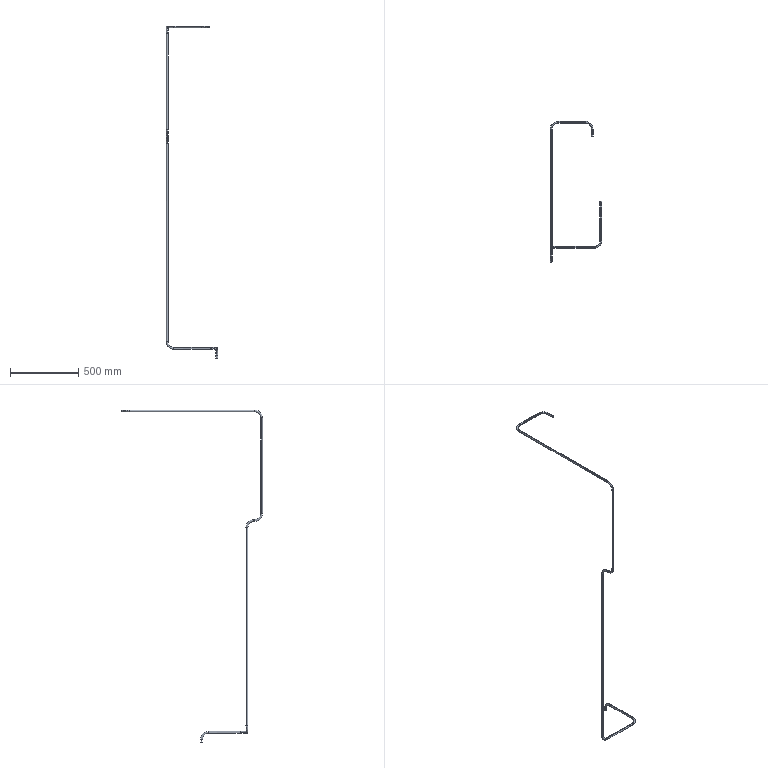Part | SolidWorks | features Sweep 5 | 1 solid | 70 faces | box 377.2 x 1030 x 2425 mm | volume 462848 mm3 | cylinder 36 | torus 32 | plane 2 | commonest cylinder face diameters 8 x18 14 x18